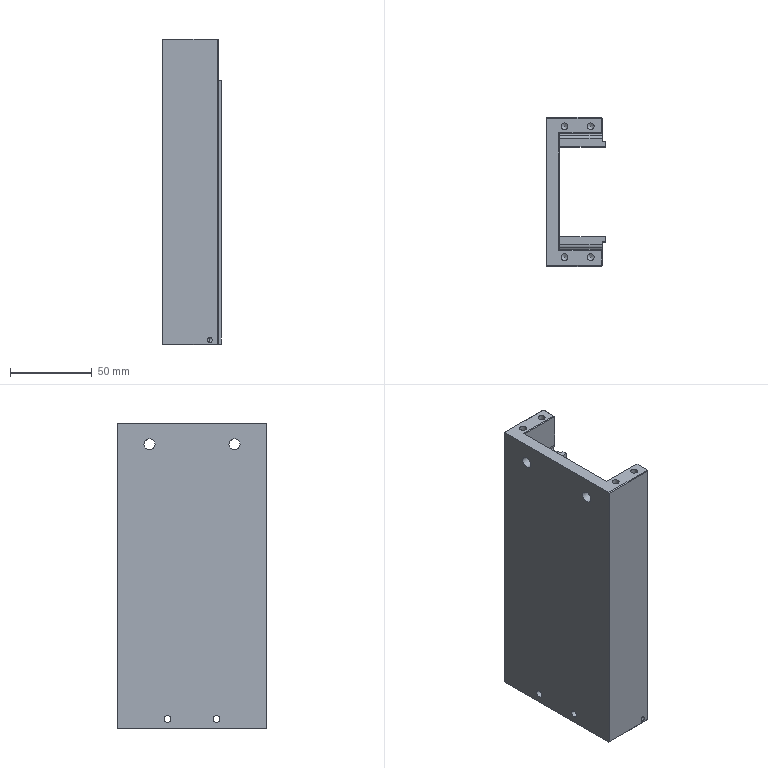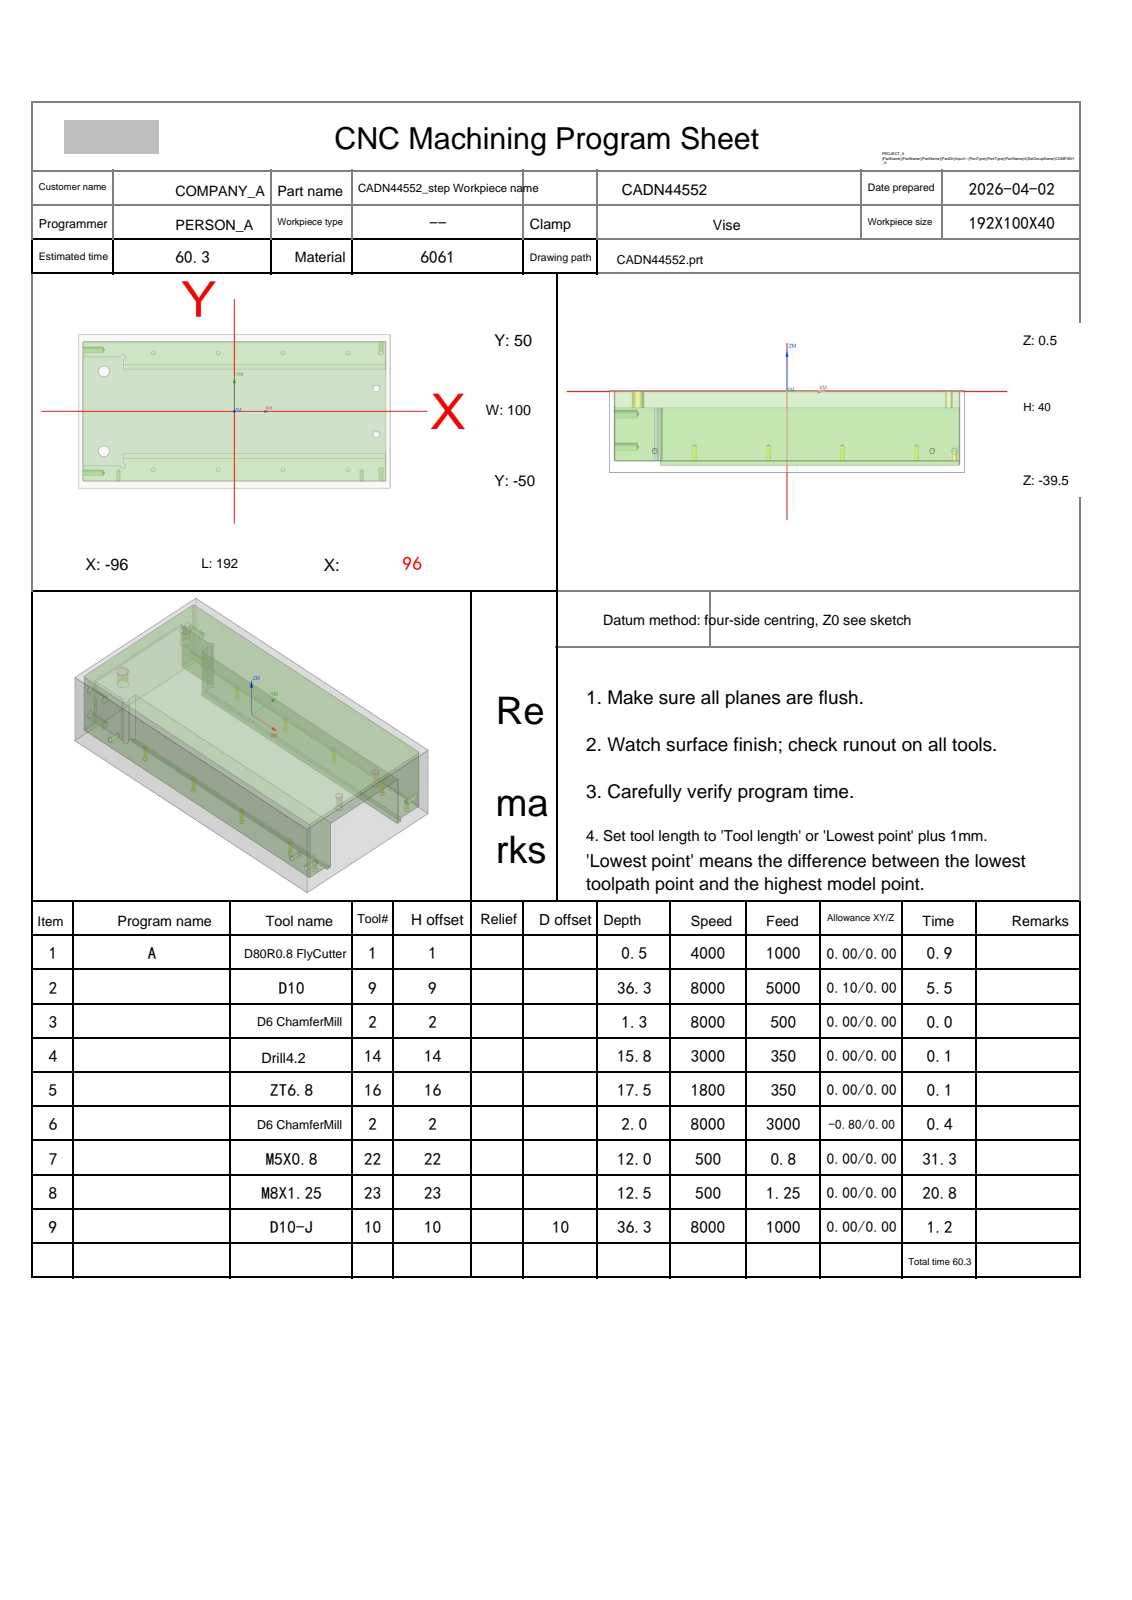NC program | NX | posted by the shop | part box 36 x 91 x 187 mm
Whole program:
%
O0001
(Machine time: 110.14 MIN)
(===Total Tool:8===)
(T1=D80R0.8 FlyCutter D=80.  R=0.8  D-  H01 Z=-0.   )
(T9=D10     D=10.  R=0.   D-  H09 Z=-35.8 )
(T2=D6 ChamferMill   D=6.   R=0.   D-  H02 Z=-1.5  )
(T14=Drill 4.2  D=4.2  DR_a=118 D-  H14 Z=-15.26)
(T16=ZT6.8  D=6.8  DR_a=118 D-  H16 Z=-17.04)
(T22=M5X0.8 D=4.2  DR_a=180 D-  H22 Z=-11.5 )
(T23=M8X1.25 D=6.8  DR_a=180 D-  H23 Z=-12.  )
(T10=D10-J  D=10.  R=0.   D10 H10 Z=-35.8 )
G80 G90 G17 G49 G40
G91 G28 Z0
M01
N1 T01 M06
(D80R0.8 FlyCutter  D=80. R=0.8 H=01 ce=0.00 di=0.00)
G00 G90 G54 X138.5 Y-42.75 M03 S4000
G43 H01 Z20.
M08
Z2.
G01 Z0.0 F1000.
X133.5
X-133.5
Y0.0
X133.5
Y42.75
X-133.5
X-138.5
Z2.
G00 Z20.
G91 G28 Z0.0
M05
M09
G91 G28 Z0.0
M01
N2 T09 M06
(D10  D=10. R=0. H=09 ce=0.10 di=0.00)
G00 G90 G54 X0.0 Y-50.6 M03 S8000
G43 H09 Z20.
M08
Z.5
G01 X-93. Z.375 F5000.
G02 X-96.606 Y-49.106 Z.37 I0.0 J5.1
G01 X-97.106 Y-48.606 Z.369
G02 X-98.6 Y-45. Z.363 I3.606 J3.606
G01 Y45. Z.242
G02 X-97.106 Y48.606 Z.237 I5.1 J0.0
G01 X-96.606 Y49.106 Z.236
G02 X-93. Y50.6 Z.23 I3.606 J-3.606
G01 X93. Z-.02
G02 X96.606 Y49.106 Z-.025 I0.0 J-5.1
G01 X97.106 Y48.606 Z-.026
G02 X98.6 Y45. Z-.031 I-3.606 J-3.606
G01 Y-45. Z-.152
G02 X97.106 Y-48.606 Z-.158 I-5.1 J0.0
G01 X96.606 Y-49.106 Z-.159
G02 X93. Y-50.6 Z-.164 I-3.606 J3.606
G01 X-93. Z-.414
G02 X-96.606 Y-49.106 Z-.42 I0.0 J5.1
G01 X-97.106 Y-48.606 Z-.421
G02 X-98.6 Y-45. Z-.426 I3.606 J3.606
G01 Y45. Z-.547
G02 X-97.106 Y48.606 Z-.552 I5.1 J0.0
G01 X-96.606 Y49.106 Z-.553
G02 X-93. Y50.6 Z-.559 I3.606 J-3.606
G01 X93. Z-.809
G02 X96.606 Y49.106 Z-.814 I0.0 J-5.1
G01 X97.106 Y48.606 Z-.815
G02 X98.6 Y45. Z-.82 I-3.606 J-3.606
G01 Y-45. Z-.941
G02 X97.106 Y-48.606 Z-.947 I-5.1 J0.0
G01 X96.606 Y-49.106 Z-.948
G02 X93. Y-50.6 Z-.953 I-3.606 J3.606
G01 X-93. Z-1.203
G02 X-96.606 Y-49.106 Z-1.209 I0.0 J5.1
G01 X-97.106 Y-48.606 Z-1.21
G02 X-98.6 Y-45. Z-1.215 I3.606 J3.606
G01 Y45. Z-1.336
G02 X-97.106 Y48.606 Z-1.341 I5.1 J0.0
G01 X-96.606 Y49.106 Z-1.342
G02 X-93. Y50.6 Z-1.348 I3.606 J-3.606
G01 X93. Z-1.598
G02 X96.606 Y49.106 Z-1.603 I0.0 J-5.1
G01 X97.106 Y48.606 Z-1.604
G02 X98.6 Y45. Z-1.61 I-3.606 J-3.606
G01 Y-45. Z-1.731
G02 X97.106 Y-48.606 Z-1.736 I-5.1 J0.0
G01 X96.606 Y-49.106 Z-1.737
G02 X93. Y-50.6 Z-1.742 I-3.606 J3.606
G01 X-93. Z-1.992
G02 X-96.606 Y-49.106 Z-1.998 I0.0 J5.1
G01 X-97.106 Y-48.606 Z-1.999
G02 X-98.6 Y-45. Z-2.004 I3.606 J3.606
G01 Y45. Z-2.125
G02 X-97.106 Y48.606 Z-2.131 I5.1 J0.0
G01 X-96.606 Y49.106 Z-2.132
G02 X-93. Y50.6 Z-2.137 I3.606 J-3.606
G01 X93. Z-2.387
G02 X96.606 Y49.106 Z-2.392 I0.0 J-5.1
G01 X97.106 Y48.606 Z-2.393
G02 X98.6 Y45. Z-2.399 I-3.606 J-3.606
G01 Y-45. Z-2.52
G02 X97.106 Y-48.606 Z-2.525 I-5.1 J0.0
G01 X96.606 Y-49.106 Z-2.526
G02 X93. Y-50.6 Z-2.531 I-3.606 J3.606
G01 X-93. Z-2.782
G02 X-96.606 Y-49.106 Z-2.787 I0.0 J5.1
G01 X-97.106 Y-48.606 Z-2.788
G02 X-98.6 Y-45. Z-2.793 I3.606 J3.606
G01 Y45. Z-2.914
G02 X-97.106 Y48.606 Z-2.92 I5.1 J0.0
G01 X-96.606 Y49.106 Z-2.921
G02 X-93. Y50.6 Z-2.926 I3.606 J-3.606
G01 X93. Z-3.176
G02 X96.606 Y49.106 Z-3.182 I0.0 J-5.1
G01 X97.106 Y48.606
G02 X98.6 Y45. Z-3.188 I-3.606 J-3.606
G01 Y-45. Z-3.309
G02 X97.106 Y-48.606 Z-3.314 I-5.1 J0.0
G01 X96.606 Y-49.106 Z-3.315
G02 X93. Y-50.6 Z-3.321 I-3.606 J3.606
G01 X-93. Z-3.571
G02 X-96.606 Y-49.106 Z-3.576 I0.0 J5.1
G01 X-97.106 Y-48.606 Z-3.577
G02 X-98.6 Y-45. Z-3.582 I3.606 J3.606
G01 Y45. Z-3.703
G02 X-97.106 Y48.606 Z-3.709 I5.1 J0.0
G01 X-96.606 Y49.106 Z-3.71
G02 X-93. Y50.6 Z-3.715 I3.606 J-3.606
G01 X93. Z-3.965
G02 X96.606 Y49.106 Z-3.971 I0.0 J-5.1
G01 X97.106 Y48.606 Z-3.972
G02 X98.6 Y45. Z-3.977 I-3.606 J-3.606
G01 Y-45. Z-4.098
G02 X97.106 Y-48.606 Z-4.103 I-5.1 J0.0
G01 X96.606 Y-49.106 Z-4.104
G02 X93. Y-50.6 Z-4.11 I-3.606 J3.606
G01 X-93. Z-4.36
G02 X-96.606 Y-49.106 Z-4.365 I0.0 J5.1
G01 X-97.106 Y-48.606 Z-4.366
G02 X-98.6 Y-45. Z-4.372 I3.606 J3.606
G01 Y45. Z-4.493
G02 X-97.106 Y48.606 Z-4.498 I5.1 J0.0
G01 X-96.606 Y49.106 Z-4.499
G02 X-93. Y50.6 Z-4.504 I3.606 J-3.606
G01 X93. Z-4.754
G02 X96.606 Y49.106 Z-4.76 I0.0 J-5.1
G01 X97.106 Y48.606 Z-4.761
G02 X98.6 Y45. Z-4.766 I-3.606 J-3.606
G01 Y-45. Z-4.887
G02 X97.106 Y-48.606 Z-4.893 I-5.1 J0.0
G01 X96.606 Y-49.106
G02 X93. Y-50.6 Z-4.899 I-3.606 J3.606
G01 X-93. Z-5.149
G02 X-96.606 Y-49.106 Z-5.154 I0.0 J5.1
G01 X-97.106 Y-48.606 Z-5.155
G02 X-98.6 Y-45. Z-5.161 I3.606 J3.606
G01 Y45. Z-5.282
G02 X-97.106 Y48.606 Z-5.287 I5.1 J0.0
G01 X-96.606 Y49.106 Z-5.288
G02 X-93. Y50.6 Z-5.293 I3.606 J-3.606
G01 X93. Z-5.544
G02 X96.606 Y49.106 Z-5.549 I0.0 J-5.1
G01 X97.106 Y48.606 Z-5.55
G02 X98.6 Y45. Z-5.555 I-3.606 J-3.606
G01 Y-45. Z-5.676
G02 X97.106 Y-48.606 Z-5.682 I-5.1 J0.0
G01 X96.606 Y-49.106 Z-5.683
G02 X93. Y-50.6 Z-5.688 I-3.606 J3.606
G01 X-93. Z-5.938
G02 X-96.606 Y-49.106 Z-5.943 I0.0 J5.1
G01 X-97.106 Y-48.606 Z-5.944
G02 X-98.6 Y-45. Z-5.95 I3.606 J3.606
G01 Y45. Z-6.071
G02 X-97.106 Y48.606 Z-6.076 I5.1 J0.0
G01 X-96.606 Y49.106 Z-6.077
G02 X-93. Y50.6 Z-6.083 I3.606 J-3.606
G01 X93. Z-6.333
G02 X96.606 Y49.106 Z-6.338 I0.0 J-5.1
G01 X97.106 Y48.606 Z-6.339
G02 X98.6 Y45. Z-6.344 I-3.606 J-3.606
G01 Y-45. Z-6.465
G02 X97.106 Y-48.606 Z-6.471 I-5.1 J0.0
G01 X96.606 Y-49.106 Z-6.472
G02 X93. Y-50.6 Z-6.477 I-3.606 J3.606
G01 X-93. Z-6.727
G02 X-96.606 Y-49.106 Z-6.733 I0.0 J5.1
G01 X-97.106 Y-48.606 Z-6.734
G02 X-98.6 Y-45. Z-6.739 I3.606 J3.606
G01 Y45. Z-6.86
G02 X-97.106 Y48.606 Z-6.865 I5.1 J0.0
G01 X-96.606 Y49.106 Z-6.866
G02 X-93. Y50.6 Z-6.872 I3.606 J-3.606
G01 X93. Z-7.122
G02 X96.606 Y49.106 Z-7.127 I0.0 J-5.1
G01 X97.106 Y48.606 Z-7.128
G02 X98.6 Y45. Z-7.134 I-3.606 J-3.606
G01 Y-45. Z-7.255
G02 X97.106 Y-48.606 Z-7.26 I-5.1 J0.0
G01 X96.606 Y-49.106 Z-7.261
G02 X93. Y-50.6 Z-7.266 I-3.606 J3.606
G01 X-93. Z-7.516
G02 X-96.606 Y-49.106 Z-7.522 I0.0 J5.1
G01 X-97.106 Y-48.606 Z-7.523
G02 X-98.6 Y-45. Z-7.528 I3.606 J3.606
G01 Y45. Z-7.649
G02 X-97.106 Y48.606 Z-7.654 I5.1 J0.0
G01 X-96.606 Y49.106 Z-7.655
G02 X-93. Y50.6 Z-7.661 I3.606 J-3.606
G01 X93. Z-7.911
G02 X96.606 Y49.106 Z-7.916 I0.0 J-5.1
G01 X97.106 Y48.606 Z-7.917
G02 X98.6 Y45. Z-7.923 I-3.606 J-3.606
G01 Y-45. Z-8.044
G02 X97.106 Y-48.606 Z-8.049 I-5.1 J0.0
G01 X96.606 Y-49.106 Z-8.05
G02 X93. Y-50.6 Z-8.055 I-3.606 J3.606
G01 X-93. Z-8.305
G02 X-96.606 Y-49.106 Z-8.311 I0.0 J5.1
G01 X-97.106 Y-48.606 Z-8.312
G02 X-98.6 Y-45. Z-8.317 I3.606 J3.606
G01 Y45. Z-8.438
G02 X-97.106 Y48.606 Z-8.444 I5.1 J0.0
G01 X-96.606 Y49.106 Z-8.445
G02 X-93. Y50.6 Z-8.45 I3.606 J-3.606
G01 X93. Z-8.7
G02 X96.606 Y49.106 Z-8.705 I0.0 J-5.1
G01 X97.106 Y48.606 Z-8.706
G02 X98.6 Y45. Z-8.712 I-3.606 J-3.606
G01 Y-45. Z-8.833
G02 X97.106 Y-48.606 Z-8.838 I-5.1 J0.0
G01 X96.606 Y-49.106 Z-8.839
G02 X93. Y-50.6 Z-8.845 I-3.606 J3.606
G01 X-93. Z-9.095
G02 X-96.606 Y-49.106 Z-9.1 I0.0 J5.1
G01 X-97.106 Y-48.606 Z-9.101
G02 X-98.6 Y-45. Z-9.106 I3.606 J3.606
G01 Y45. Z-9.227
G02 X-97.106 Y48.606 Z-9.233 I5.1 J0.0
G01 X-96.606 Y49.106 Z-9.234
G02 X-93. Y50.6 Z-9.239 I3.606 J-3.606
G01 X93. Z-9.489
G02 X96.606 Y49.106 Z-9.495 I0.0 J-5.1
G01 X97.106 Y48.606 Z-9.496
G02 X98.6 Y45. Z-9.501 I-3.606 J-3.606
G01 Y-45. Z-9.622
G02 X97.106 Y-48.606 Z-9.627 I-5.1 J0.0
G01 X96.606 Y-49.106 Z-9.628
G02 X93. Y-50.6 Z-9.634 I-3.606 J3.606
G01 X-93. Z-9.884
G02 X-96.606 Y-49.106 Z-9.889 I0.0 J5.1
G01 X-97.106 Y-48.606 Z-9.89
G02 X-98.6 Y-45. Z-9.895 I3.606 J3.606
G01 Y45. Z-10.016
G02 X-97.106 Y48.606 Z-10.022 I5.1 J0.0
G01 X-96.606 Y49.106 Z-10.023
G02 X-93. Y50.6 Z-10.028 I3.606 J-3.606
G01 X93. Z-10.278
G02 X96.606 Y49.106 Z-10.284 I0.0 J-5.1
G01 X97.106 Y48.606 Z-10.285
G02 X98.6 Y45. Z-10.29 I-3.606 J-3.606
G01 Y-45. Z-10.411
G02 X97.106 Y-48.606 Z-10.416 I-5.1 J0.0
G01 X96.606 Y-49.106 Z-10.417
G02 X93. Y-50.6 Z-10.423 I-3.606 J3.606
G01 X-93. Z-10.673
G02 X-96.606 Y-49.106 Z-10.678 I0.0 J5.1
G01 X-97.106 Y-48.606 Z-10.679
G02 X-98.6 Y-45. Z-10.685 I3.606 J3.606
G01 Y45. Z-10.806
G02 X-97.106 Y48.606 Z-10.811 I5.1 J0.0
G01 X-96.606 Y49.106 Z-10.812
G02 X-93. Y50.6 Z-10.817 I3.606 J-3.606
G01 X93. Z-11.067
G02 X96.606 Y49.106 Z-11.073 I0.0 J-5.1
G01 X97.106 Y48.606 Z-11.074
G02 X98.6 Y45. Z-11.079 I-3.606 J-3.606
G01 Y-45. Z-11.2
G02 X97.106 Y-48.606 Z-11.206 I-5.1 J0.0
G01 X96.606 Y-49.106 Z-11.207
G02 X93. Y-50.6 Z-11.212 I-3.606 J3.606
G01 X-93. Z-11.462
G02 X-96.606 Y-49.106 Z-11.467 I0.0 J5.1
G01 X-97.106 Y-48.606 Z-11.468
G02 X-98.6 Y-45. Z-11.474 I3.606 J3.606
G01 Y45. Z-11.595
G02 X-97.106 Y48.606 Z-11.6 I5.1 J0.0
G01 X-96.606 Y49.106 Z-11.601
G02 X-93. Y50.6 Z-11.606 I3.606 J-3.606
G01 X93. Z-11.857
G02 X96.606 Y49.106 Z-11.862 I0.0 J-5.1
G01 X97.106 Y48.606 Z-11.863
G02 X98.6 Y45. Z-11.868 I-3.606 J-3.606
G01 Y-45. Z-11.989
G02 X97.106 Y-48.606 Z-11.995 I-5.1 J0.0
G01 X96.606 Y-49.106 Z-11.996
G02 X93. Y-50.6 Z-12.001 I-3.606 J3.606
G01 X-93. Z-12.251
G02 X-96.606 Y-49.106 Z-12.257 I0.0 J5.1
G01 X-97.106 Y-48.606
G02 X-98.6 Y-45. Z-12.263 I3.606 J3.606
G01 Y45. Z-12.384
G02 X-97.106 Y48.606 Z-12.389 I5.1 J0.0
G01 X-96.606 Y49.106 Z-12.39
G02 X-93. Y50.6 Z-12.396 I3.606 J-3.606
G01 X93. Z-12.646
G02 X96.606 Y49.106 Z-12.651 I0.0 J-5.1
G01 X97.106 Y48.606 Z-12.652
G02 X98.6 Y45. Z-12.657 I-3.606 J-3.606
G01 Y-45. Z-12.778
G02 X97.106 Y-48.606 Z-12.784 I-5.1 J0.0
G01 X96.606 Y-49.106 Z-12.785
G02 X93. Y-50.6 Z-12.79 I-3.606 J3.606
G01 X-93. Z-13.04
G02 X-96.606 Y-49.106 Z-13.046 I0.0 J5.1
G01 X-97.106 Y-48.606 Z-13.047
G02 X-98.6 Y-45. Z-13.052 I3.606 J3.606
G01 Y45. Z-13.173
G02 X-97.106 Y48.606 Z-13.178 I5.1 J0.0
G01 X-96.606 Y49.106 Z-13.179
G02 X-93. Y50.6 Z-13.185 I3.606 J-3.606
G01 X93. Z-13.435
G02 X96.606 Y49.106 Z-13.44 I0.0 J-5.1
G01 X97.106 Y48.606 Z-13.441
G02 X98.6 Y45. Z-13.447 I-3.606 J-3.606
G01 Y-45. Z-13.568
G02 X97.106 Y-48.606 Z-13.573 I-5.1 J0.0
G01 X96.606 Y-49.106 Z-13.574
G02 X93. Y-50.6 Z-13.579 I-3.606 J3.606
G01 X-93. Z-13.829
G02 X-96.606 Y-49.106 Z-13.835 I0.0 J5.1
G01 X-97.106 Y-48.606 Z-13.836
G02 X-98.6 Y-45. Z-13.841 I3.606 J3.606
G01 Y45. Z-13.962
G02 X-97.106 Y48.606 Z-13.968 I5.1 J0.0
G01 X-96.606 Y49.106
G02 X-93. Y50.6 Z-13.974 I3.606 J-3.606
G01 X93. Z-14.224
G02 X96.606 Y49.106 Z-14.229 I0.0 J-5.1
G01 X97.106 Y48.606 Z-14.23
G02 X98.6 Y45. Z-14.236 I-3.606 J-3.606
G01 Y-45. Z-14.357
G02 X97.106 Y-48.606 Z-14.362 I-5.1 J0.0
G01 X96.606 Y-49.106 Z-14.363
G02 X93. Y-50.6 Z-14.368 I-3.606 J3.606
G01 X-93. Z-14.619
G02 X-96.606 Y-49.106 Z-14.624 I0.0 J5.1
G01 X-97.106 Y-48.606 Z-14.625
G02 X-98.6 Y-45. Z-14.63 I3.606 J3.606
G01 Y45. Z-14.751
G02 X-97.106 Y48.606 Z-14.757 I5.1 J0.0
G01 X-96.606 Y49.106 Z-14.758
G02 X-93. Y50.6 Z-14.763 I3.606 J-3.606
G01 X93. Z-15.013
G02 X96.606 Y49.106 Z-15.018 I0.0 J-5.1
G01 X97.106 Y48.606 Z-15.019
G02 X98.6 Y45. Z-15.025 I-3.606 J-3.606
G01 Y-45. Z-15.146
G02 X97.106 Y-48.606 Z-15.151 I-5.1 J0.0
G01 X96.606 Y-49.106 Z-15.152
G02 X93. Y-50.6 Z-15.158 I-3.606 J3.606
G01 X-93. Z-15.408
G02 X-96.606 Y-49.106 Z-15.413 I0.0 J5.1
G01 X-97.106 Y-48.606 Z-15.414
G02 X-98.6 Y-45. Z-15.419 I3.606 J3.606
G01 Y45. Z-15.54
G02 X-97.106 Y48.606 Z-15.546 I5.1 J0.0
G01 X-96.606 Y49.106 Z-15.547
G02 X-93. Y50.6 Z-15.552 I3.606 J-3.606
G01 X93. Z-15.802
G02 X96.606 Y49.106 Z-15.808 I0.0 J-5.1
G01 X97.106 Y48.606 Z-15.809
G02 X98.6 Y45. Z-15.814 I-3.606 J-3.606
G01 Y-45. Z-15.935
G02 X97.106 Y-48.606 Z-15.94 I-5.1 J0.0
G01 X96.606 Y-49.106 Z-15.941
G02 X93. Y-50.6 Z-15.947 I-3.606 J3.606
G01 X-93. Z-16.197
G02 X-96.606 Y-49.106 Z-16.202 I0.0 J5.1
G01 X-97.106 Y-48.606 Z-16.203
G02 X-98.6 Y-45. Z-16.209 I3.606 J3.606
G01 Y45. Z-16.33
G02 X-97.106 Y48.606 Z-16.335 I5.1 J0.0
G01 X-96.606 Y49.106 Z-16.336
G02 X-93. Y50.6 Z-16.341 I3.606 J-3.606
G01 X93. Z-16.591
G02 X96.606 Y49.106 Z-16.597 I0.0 J-5.1
G01 X97.106 Y48.606 Z-16.598
G02 X98.6 Y45. Z-16.603 I-3.606 J-3.606
G01 Y-45. Z-16.724
G02 X97.106 Y-48.606 Z-16.729 I-5.1 J0.0
G01 X96.606 Y-49.106 Z-16.73
G02 X93. Y-50.6 Z-16.736 I-3.606 J3.606
G01 X-93. Z-16.986
G02 X-96.606 Y-49.106 Z-16.991 I0.0 J5.1
G01 X-97.106 Y-48.606 Z-16.992
G02 X-98.6 Y-45. Z-16.998 I3.606 J3.606
G01 Y45. Z-17.119
G02 X-97.106 Y48.606 Z-17.124 I5.1 J0.0
G01 X-96.606 Y49.106 Z-17.125
G02 X-93. Y50.6 Z-17.13 I3.606 J-3.606
G01 X93. Z-17.38
G02 X96.606 Y49.106 Z-17.386 I0.0 J-5.1
G01 X97.106 Y48.606 Z-17.387
G02 X98.6 Y45. Z-17.392 I-3.606 J-3.606
G01 Y-45. Z-17.513
G02 X97.106 Y-48.606 Z-17.519 I-5.1 J0.0
G01 X96.606 Y-49.106 Z-17.52
G02 X93. Y-50.6 Z-17.525 I-3.606 J3.606
G01 X-93. Z-17.775
G02 X-96.606 Y-49.106 Z-17.78 I0.0 J5.1
G01 X-97.106 Y-48.606 Z-17.781
G02 X-98.6 Y-45. Z-17.787 I3.606 J3.606
G01 Y45. Z-17.908
G02 X-97.106 Y48.606 Z-17.913 I5.1 J0.0
G01 X-96.606 Y49.106 Z-17.914
G02 X-93. Y50.6 Z-17.92 I3.606 J-3.606
G01 X93. Z-18.17
G02 X96.606 Y49.106 Z-18.175 I0.0 J-5.1
G01 X97.106 Y48.606 Z-18.176
G02 X98.6 Y45. Z-18.181 I-3.606 J-3.606
G01 Y-45. Z-18.302
G02 X97.106 Y-48.606 Z-18.308 I-5.1 J0.0
G01 X96.606 Y-49.106 Z-18.309
G02 X93. Y-50.6 Z-18.314 I-3.606 J3.606
G01 X-93. Z-18.564
G02 X-96.606 Y-49.106 Z-18.57 I0.0 J5.1
G01 X-97.106 Y-48.606 Z-18.571
G02 X-98.6 Y-45. Z-18.576 I3.606 J3.606
G01 Y45. Z-18.697
G02 X-97.106 Y48.606 Z-18.702 I5.1 J0.0
G01 X-96.606 Y49.106 Z-18.703
G02 X-93. Y50.6 Z-18.709 I3.606 J-3.606
G01 X93. Z-18.959
G02 X96.606 Y49.106 Z-18.964 I0.0 J-5.1
G01 X97.106 Y48.606 Z-18.965
G02 X98.6 Y45. Z-18.97 I-3.606 J-3.606
G01 Y-45. Z-19.091
G02 X97.106 Y-48.606 Z-19.097 I-5.1 J0.0
G01 X96.606 Y-49.106 Z-19.098
G02 X93. Y-50.6 Z-19.103 I-3.606 J3.606
G01 X-93. Z-19.353
G02 X-96.606 Y-49.106 Z-19.359 I0.0 J5.1
G01 X-97.106 Y-48.606 Z-19.36
G02 X-98.6 Y-45. Z-19.365 I3.606 J3.606
G01 Y45. Z-19.486
G02 X-97.106 Y48.606 Z-19.491 I5.1 J0.0
G01 X-96.606 Y49.106 Z-19.492
G02 X-93. Y50.6 Z-19.498 I3.606 J-3.606
G01 X93. Z-19.748
G02 X96.606 Y49.106 Z-19.753 I0.0 J-5.1
G01 X97.106 Y48.606 Z-19.754
G02 X98.6 Y45. Z-19.76 I-3.606 J-3.606
G01 Y-45. Z-19.881
G02 X97.106 Y-48.606 Z-19.886 I-5.1 J0.0
G01 X96.606 Y-49.106 Z-19.887
G02 X93. Y-50.6 Z-19.892 I-3.606 J3.606
G01 X-93. Z-20.142
G02 X-96.606 Y-49.106 Z-20.148 I0.0 J5.1
G01 X-97.106 Y-48.606 Z-20.149
G02 X-98.6 Y-45. Z-20.154 I3.606 J3.606
G01 Y45. Z-20.275
G02 X-97.106 Y48.606 Z-20.281 I5.1 J0.0
G01 X-96.606 Y49.106 Z-20.282
G02 X-93. Y50.6 Z-20.287 I3.606 J-3.606
G01 X93. Z-20.537
G02 X96.606 Y49.106 Z-20.542 I0.0 J-5.1
G01 X97.106 Y48.606 Z-20.543
G02 X98.6 Y45. Z-20.549 I-3.606 J-3.606
G01 Y-45. Z-20.67
G02 X97.106 Y-48.606 Z-20.675 I-5.1 J0.0
G01 X96.606 Y-49.106 Z-20.676
G02 X93. Y-50.6 Z-20.681 I-3.606 J3.606
G01 X-93. Z-20.932
G02 X-96.606 Y-49.106 Z-20.937 I0.0 J5.1
G01 X-97.106 Y-48.606 Z-20.938
G02 X-98.6 Y-45. Z-20.943 I3.606 J3.606
G01 Y45. Z-21.064
G02 X-97.106 Y48.606 Z-21.07 I5.1 J0.0
G01 X-96.606 Y49.106 Z-21.071
G02 X-93. Y50.6 Z-21.076 I3.606 J-3.606
G01 X93. Z-21.326
G02 X96.606 Y49.106 Z-21.332 I0.0 J-5.1
G01 X97.106 Y48.606
G02 X98.6 Y45. Z-21.338 I-3.606 J-3.606
G01 Y-45. Z-21.459
G02 X97.106 Y-48.606 Z-21.464 I-5.1 J0.0
G01 X96.606 Y-49.106 Z-21.465
G02 X93. Y-50.6 Z-21.471 I-3.606 J3.606
G01 X-93. Z-21.721
G02 X-96.606 Y-49.106 Z-21.726 I0.0 J5.1
G01 X-97.106 Y-48.606 Z-21.727
G02 X-98.6 Y-45. Z-21.732 I3.606 J3.606
G01 Y45. Z-21.853
G02 X-97.106 Y48.606 Z-21.859 I5.1 J0.0
G01 X-96.606 Y49.106 Z-21.86
G02 X-93. Y50.6 Z-21.865 I3.606 J-3.606
G01 X93. Z-22.115
G02 X96.606 Y49.106 Z-22.121 I0.0 J-5.1
G01 X97.106 Y48.606 Z-22.122
G02 X98.6 Y45. Z-22.127 I-3.606 J-3.606
G01 Y-45. Z-22.248
G02 X97.106 Y-48.606 Z-22.253 I-5.1 J0.0
G01 X96.606 Y-49.106 Z-22.254
G02 X93. Y-50.6 Z-22.26 I-3.606 J3.606
G01 X-93. Z-22.51
G02 X-96.606 Y-49.106 Z-22.515 I0.0 J5.1
G01 X-97.106 Y-48.606 Z-22.516
G02 X-98.6 Y-45. Z-22.522 I3.606 J3.606
G01 Y45. Z-22.643
G02 X-97.106 Y48.606 Z-22.648 I5.1 J0.0
G01 X-96.606 Y49.106 Z-22.649
G02 X-93. Y50.6 Z-22.654 I3.606 J-3.606
G01 X93. Z-22.904
G02 X96.606 Y49.106 Z-22.91 I0.0 J-5.1
G01 X97.106 Y48.606 Z-22.911
G02 X98.6 Y45. Z-22.916 I-3.606 J-3.606
G01 Y-45. Z-23.037
G02 X97.106 Y-48.606 Z-23.043 I-5.1 J0.0
G01 X96.606 Y-49.106
G02 X93. Y-50.6 Z-23.049 I-3.606 J3.606
G01 X-93. Z-23.299
G02 X-96.606 Y-49.106 Z-23.304 I0.0 J5.1
G01 X-97.106 Y-48.606 Z-23.305
G02 X-98.6 Y-45. Z-23.311 I3.606 J3.606
G01 Y45. Z-23.432
G02 X-97.106 Y48.606 Z-23.437 I5.1 J0.0
G01 X-96.606 Y49.106 Z-23.438
G02 X-93. Y50.6 Z-23.443 I3.606 J-3.606
G01 X93. Z-23.694
G02 X96.606 Y49.106 Z-23.699 I0.0 J-5.1
G01 X97.106 Y48.606 Z-23.7
G02 X98.6 Y45. Z-23.705 I-3.606 J-3.606
G01 Y-45. Z-23.826
G02 X97.106 Y-48.606 Z-23.832 I-5.1 J0.0
G01 X96.606 Y-49.106 Z-23.833
G02 X93. Y-50.6 Z-23.838 I-3.606 J3.606
G01 X-93. Z-24.088
G02 X-96.606 Y-49.106 Z-24.093 I0.0 J5.1
G01 X-97.106 Y-48.606 Z-24.094
G02 X-98.6 Y-45. Z-24.1 I3.606 J3.606
G01 Y45. Z-24.221
G02 X-97.106 Y48.606 Z-24.226 I5.1 J0.0
G01 X-96.606 Y49.106 Z-24.227
G02 X-93. Y50.6 Z-24.233 I3.606 J-3.606
G01 X93. Z-24.483
G02 X96.606 Y49.106 Z-24.488 I0.0 J-5.1
G01 X97.106 Y48.606 Z-24.489
G02 X98.6 Y45. Z-24.494 I-3.606 J-3.606
G01 Y-45. Z-24.615
G02 X97.106 Y-48.606 Z-24.621 I-5.1 J0.0
G01 X96.606 Y-49.106 Z-24.622
G02 X93. Y-50.6 Z-24.627 I-3.606 J3.606
G01 X-93. Z-24.877
G02 X-96.606 Y-49.106 Z-24.883 I0.0 J5.1
G01 X-97.106 Y-48.606 Z-24.884
G02 X-98.6 Y-45. Z-24.889 I3.606 J3.606
G01 Y45. Z-25.01
G02 X-97.106 Y48.606 Z-25.015 I5.1 J0.0
G01 X-96.606 Y49.106 Z-25.016
G02 X-93. Y50.6 Z-25.022 I3.606 J-3.606
G01 X93. Z-25.272
G02 X96.606 Y49.106 Z-25.277 I0.0 J-5.1
G01 X97.106 Y48.606 Z-25.278
G02 X98.6 Y45. Z-25.284 I-3.606 J-3.606
G01 Y-45. Z-25.405
G02 X97.106 Y-48.606 Z-25.41 I-5.1 J0.0
G01 X96.606 Y-49.106 Z-25.411
G02 X93. Y-50.6 Z-25.416 I-3.606 J3.606
G01 X-93. Z-25.666
G02 X-96.606 Y-49.106 Z-25.672 I0.0 J5.1
G01 X-97.106 Y-48.606 Z-25.673
G02 X-98.6 Y-45. Z-25.678 I3.606 J3.606
G01 Y45. Z-25.799
G02 X-97.106 Y48.606 Z-25.804 I5.1 J0.0
G01 X-96.606 Y49.106 Z-25.805
G02 X-93. Y50.6 Z-25.811 I3.606 J-3.606
G01 X93. Z-26.061
G02 X96.606 Y49.106 Z-26.066 I0.0 J-5.1
G01 X97.106 Y48.606 Z-26.067
G02 X98.6 Y45. Z-26.073 I-3.606 J-3.606
G01 Y-45. Z-26.194
G02 X97.106 Y-48.606 Z-26.199 I-5.1 J0.0
G01 X96.606 Y-49.106 Z-26.2
G02 X93. Y-50.6 Z-26.205 I-3.606 J3.606
G01 X-93. Z-26.455
G02 X-96.606 Y-49.106 Z-26.461 I0.0 J5.1
G01 X-97.106 Y-48.606 Z-26.462
G02 X-98.6 Y-45. Z-26.467 I3.606 J3.606
G01 Y45. Z-26.588
G02 X-97.106 Y48.606 Z-26.594 I5.1 J0.0
G01 X-96.606 Y49.106 Z-26.595
G02 X-93. Y50.6 Z-26.6 I3.606 J-3.606
G01 X93. Z-26.85
G02 X96.606 Y49.106 Z-26.855 I0.0 J-5.1
G01 X97.106 Y48.606 Z-26.856
G02 X98.6 Y45. Z-26.862 I-3.606 J-3.606
G01 Y-45. Z-26.983
G02 X97.106 Y-48.606 Z-26.988 I-5.1 J0.0
G01 X96.606 Y-49.106 Z-26.989
G02 X93. Y-50.6 Z-26.995 I-3.606 J3.606
G01 X-93. Z-27.245
G02 X-96.606 Y-49.106 Z-27.25 I0.0 J5.1
G01 X-97.106 Y-48.606 Z-27.251
G02 X-98.6 Y-45. Z-27.256 I3.606 J3.606
G01 Y45. Z-27.377
G02 X-97.106 Y48.606 Z-27.383 I5.1 J0.0
G01 X-96.606 Y49.106 Z-27.384
G02 X-93. Y50.6 Z-27.389 I3.606 J-3.606
G01 X93. Z-27.639
G02 X96.606 Y49.106 Z-27.645 I0.0 J-5.1
G01 X97.106 Y48.606 Z-27.646
G02 X98.6 Y45. Z-27.651 I-3.606 J-3.606
G01 Y-45. Z-27.772
G02 X97.106 Y-48.606 Z-27.777 I-5.1 J0.0
G01 X96.606 Y-49.106 Z-27.778
G02 X93. Y-50.6 Z-27.784 I-3.606 J3.606
G01 X-93. Z-28.034
G02 X-96.606 Y-49.106 Z-28.039 I0.0 J5.1
G01 X-97.106 Y-48.606 Z-28.04
G02 X-98.6 Y-45. Z-28.045 I3.606 J3.606
G01 Y45. Z-28.166
G02 X-97.106 Y48.606 Z-28.172 I5.1 J0.0
G01 X-96.606 Y49.106 Z-28.173
G02 X-93. Y50.6 Z-28.178 I3.606 J-3.606
G01 X93. Z-28.428
G02 X96.606 Y49.106 Z-28.434 I0.0 J-5.1
G01 X97.106 Y48.606 Z-28.435
G02 X98.6 Y45. Z-28.44 I-3.606 J-3.606
G01 Y-45. Z-28.561
G02 X97.106 Y-48.606 Z-28.566 I-5.1 J0.0
G01 X96.606 Y-49.106 Z-28.567
G02 X93. Y-50.6 Z-28.573 I-3.606 J3.606
G01 X-93. Z-28.823
G02 X-96.606 Y-49.106 Z-28.828 I0.0 J5.1
G01 X-97.106 Y-48.606 Z-28.829
G02 X-98.6 Y-45. Z-28.835 I3.606 J3.606
G01 Y45. Z-28.956
G02 X-97.106 Y48.606 Z-28.961 I5.1 J0.0
G01 X-96.606 Y49.106 Z-28.962
G02 X-93. Y50.6 Z-28.967 I3.606 J-3.606
G01 X93. Z-29.217
G02 X96.606 Y49.106 Z-29.223 I0.0 J-5.1
G01 X97.106 Y48.606 Z-29.224
G02 X98.6 Y45. Z-29.229 I-3.606 J-3.606
G01 Y-45. Z-29.35
G02 X97.106 Y-48.606 Z-29.356 I-5.1 J0.0
G01 X96.606 Y-49.106 Z-29.357
G02 X93. Y-50.6 Z-29.362 I-3.606 J3.606
G01 X-93. Z-29.612
G02 X-96.606 Y-49.106 Z-29.617 I0.0 J5.1
G01 X-97.106 Y-48.606 Z-29.618
G02 X-98.6 Y-45. Z-29.624 I3.606 J3.606
G01 Y45. Z-29.745
G02 X-97.106 Y48.606 Z-29.75 I5.1 J0.0
G01 X-96.606 Y49.106 Z-29.751
G02 X-93. Y50.6 Z-29.756 I3.606 J-3.606
G01 X93. Z-30.007
G02 X96.606 Y49.106 Z-30.012 I0.0 J-5.1
G01 X97.106 Y48.606 Z-30.013
G02 X98.6 Y45. Z-30.018 I-3.606 J-3.606
G01 Y-45. Z-30.139
G02 X97.106 Y-48.606 Z-30.145 I-5.1 J0.0
G01 X96.606 Y-49.106 Z-30.146
G02 X93. Y-50.6 Z-30.151 I-3.606 J3.606
G01 X-93. Z-30.401
G02 X-96.606 Y-49.106 Z-30.407 I0.0 J5.1
G01 X-97.106 Y-48.606
G02 X-98.6 Y-45. Z-30.413 I3.606 J3.606
G01 Y45. Z-30.534
G02 X-97.106 Y48.606 Z-30.539 I5.1 J0.0
G01 X-96.606 Y49.106 Z-30.54
G02 X-93. Y50.6 Z-30.546 I3.606 J-3.606
G01 X93. Z-30.796
G02 X96.606 Y49.106 Z-30.801 I0.0 J-5.1
G01 X97.106 Y48.606 Z-30.802
G02 X98.6 Y45. Z-30.807 I-3.606 J-3.606
G01 Y-45. Z-30.928
G02 X97.106 Y-48.606 Z-30.934 I-5.1 J0.0
G01 X96.606 Y-49.106 Z-30.935
G02 X93. Y-50.6 Z-30.94 I-3.606 J3.606
G01 X-93. Z-31.19
G02 X-96.606 Y-49.106 Z-31.196 I0.0 J5.1
G01 X-97.106 Y-48.606 Z-31.197
G02 X-98.6 Y-45. Z-31.202 I3.606 J3.606
G01 Y45. Z-31.323
G02 X-97.106 Y48.606 Z-31.328 I5.1 J0.0
G01 X-96.606 Y49.106 Z-31.329
G02 X-93. Y50.6 Z-31.335 I3.606 J-3.606
G01 X93. Z-31.585
G02 X96.606 Y49.106 Z-31.59 I0.0 J-5.1
G01 X97.106 Y48.606 Z-31.591
G02 X98.6 Y45. Z-31.597 I-3.606 J-3.606
G01 Y-45. Z-31.718
G02 X97.106 Y-48.606 Z-31.723 I-5.1 J0.0
G01 X96.606 Y-49.106 Z-31.724
G02 X93. Y-50.6 Z-31.729 I-3.606 J3.606
G01 X-93. Z-31.979
G02 X-96.606 Y-49.106 Z-31.985 I0.0 J5.1
G01 X-97.106 Y-48.606 Z-31.986
G02 X-98.6 Y-45. Z-31.991 I3.606 J3.606
G01 Y45. Z-32.112
G02 X-97.106 Y48.606 Z-32.118 I5.1 J0.0
G01 X-96.606 Y49.106
G02 X-93. Y50.6 Z-32.124 I3.606 J-3.606
G01 X93. Z-32.374
G02 X96.606 Y49.106 Z-32.379 I0.0 J-5.1
G01 X97.106 Y48.606 Z-32.38
G02 X98.6 Y45. Z-32.386 I-3.606 J-3.606
G01 Y-45. Z-32.507
G02 X97.106 Y-48.606 Z-32.512 I-5.1 J0.0
G01 X96.606 Y-49.106 Z-32.513
G02 X93. Y-50.6 Z-32.518 I-3.606 J3.606
G01 X-93. Z-32.769
G02 X-96.606 Y-49.106 Z-32.774 I0.0 J5.1
G01 X-97.106 Y-48.606 Z-32.775
G02 X-98.6 Y-45. Z-32.78 I3.606 J3.606
G01 Y45. Z-32.901
G02 X-97.106 Y48.606 Z-32.907 I5.1 J0.0
G01 X-96.606 Y49.106 Z-32.908
G02 X-93. Y50.6 Z-32.913 I3.606 J-3.606
G01 X93. Z-33.163
G02 X96.606 Y49.106 Z-33.168 I0.0 J-5.1
G01 X97.106 Y48.606 Z-33.169
G02 X98.6 Y45. Z-33.175 I-3.606 J-3.606
G01 Y-45. Z-33.296
G02 X97.106 Y-48.606 Z-33.301 I-5.1 J0.0
G01 X96.606 Y-49.106 Z-33.302
G02 X93. Y-50.6 Z-33.308 I-3.606 J3.606
G01 X-93. Z-33.558
G02 X-96.606 Y-49.106 Z-33.563 I0.0 J5.1
G01 X-97.106 Y-48.606 Z-33.564
G02 X-98.6 Y-45. Z-33.569 I3.606 J3.606
G01 Y45. Z-33.69
G02 X-97.106 Y48.606 Z-33.696 I5.1 J0.0
G01 X-96.606 Y49.106 Z-33.697
G02 X-93. Y50.6 Z-33.702 I3.606 J-3.606
G01 X93. Z-33.952
G02 X96.606 Y49.106 Z-33.958 I0.0 J-5.1
G01 X97.106 Y48.606 Z-33.959
G02 X98.6 Y45. Z-33.964 I-3.606 J-3.606
G01 Y-45. Z-34.085
G02 X97.106 Y-48.606 Z-34.09 I-5.1 J0.0
G01 X96.606 Y-49.106 Z-34.091
G02 X93. Y-50.6 Z-34.097 I-3.606 J3.606
G01 X-93. Z-34.347
G02 X-96.606 Y-49.106 Z-34.352 I0.0 J5.1
G01 X-97.106 Y-48.606 Z-34.353
G02 X-98.6 Y-45. Z-34.359 I3.606 J3.606
G01 Y45. Z-34.48
G02 X-97.106 Y48.606 Z-34.485 I5.1 J0.0
G01 X-96.606 Y49.106 Z-34.486
G02 X-93. Y50.6 Z-34.491 I3.606 J-3.606
G01 X93. Z-34.741
G02 X96.606 Y49.106 Z-34.747 I0.0 J-5.1
G01 X97.106 Y48.606 Z-34.748
G02 X98.6 Y45. Z-34.753 I-3.606 J-3.606
G01 Y-45. Z-34.874
G02 X97.106 Y-48.606 Z-34.879 I-5.1 J0.0
G01 X96.606 Y-49.106 Z-34.88
G02 X93. Y-50.6 Z-34.886 I-3.606 J3.606
G01 X-93. Z-35.136
G02 X-96.606 Y-49.106 Z-35.141 I0.0 J5.1
G01 X-97.106 Y-48.606 Z-35.142
G02 X-98.6 Y-45. Z-35.148 I3.606 J3.606
G01 Y45. Z-35.269
G02 X-97.106 Y48.606 Z-35.274 I5.1 J0.0
G01 X-96.606 Y49.106 Z-35.275
G02 X-93. Y50.6 Z-35.28 I3.606 J-3.606
G01 X93. Z-35.53
G02 X96.606 Y49.106 Z-35.536 I0.0 J-5.1
G01 X97.106 Y48.606 Z-35.537
G02 X98.6 Y45. Z-35.542 I-3.606 J-3.606
G01 Y-45. Z-35.663
G02 X97.106 Y-48.606 Z-35.669 I-5.1 J0.0
G01 X96.606 Y-49.106 Z-35.67
G02 X93. Y-50.6 Z-35.675 I-3.606 J3.606
G01 X0.0 Z-35.8
X-93.
G02 X-96.606 Y-49.106 I0.0 J5.1
G01 X-97.106 Y-48.606
G02 X-98.6 Y-45. I3.606 J3.606
G01 Y45.
G02 X-97.106 Y48.606 I5.1 J0.0
G01 X-96.606 Y49.106
G02 X-93. Y50.6 I3.606 J-3.606
G01 X93.
G02 X96.606 Y49.106 I0.0 J-5.1
G01 X97.106 Y48.606
G02 X98.6 Y45. I-3.606 J-3.606
G01 Y-45.
G02 X97.106 Y-48.606 I-5.1 J0.0
G01 X96.606 Y-49.106
G02 X93. Y-50.6 I-3.606 J3.606
G01 X0.0
X-.5
Z-34.8
G00 Z20.
G91 G28 Z0.0
M05
M09
G91 G28 Z0.0
M01
N3 T02 M06
(D6 ChamferMill  D=6. R=0. H=02 ce=0.00 di=0.00)
G00 G90 G54 X87.5 Y-15. M03 S8000
G43 H02 Z20.
M08
G98 G81 X87.5 Y-15. Z-.8 R1. F500.
Y15.
X-80.5 Y26.
Y-26.
G80
G00 Z20.
G91 G28 Z0.0
M05
M09
G91 G28 Z0.0
M01
N4 T14 M06
(Drill 4.2 D=4.2 DR_a=118 H=14)
G00 G90 G54 X87.5 Y-15. M03 S3000
G43 H14 Z20.
M08
G98 G83 X87.5 Y-15. Z-15.262 R1. F350. Q3.
Y15.
G80
G00 Z20.
G91 G28 Z0.0
M05
M09
G91 G28 Z0.0
M01
N5 T16 M06
(ZT6.8 D=6.8 DR_a=118 H=16)
G00 G90 G54 X-80.5 Y26. M03 S1800
G43 H16 Z20.
M08
G98 G83 X-80.5 Y26. Z-17.043 R1. F350. Q3.
Y-26.
G80
G00 Z20.
G91 G28 Z0.0
M05
M09
G91 G28 Z0.0
M01
N6 T02 M06
(D6 ChamferMill  D=6. R=0. H=02 ce=0.00 di=0.00)
G00 G90 G54 X.25 Y-47.628 M03 S8000
G43 H02 Z20.
M08
Z2.099
G01 Z-1.5 F3000.
G03 X.33 Y-47.328 I-.52 J.3
X.03 Y-46.808 I-.6 J0.0
G01 X0.0 Y-46.8
X-93.
X-93.254 Y-46.775
X-93.497 Y-46.701
X-93.722 Y-46.581
X-93.919 Y-46.419
X-94.419 Y-45.919
X-94.581 Y-45.722
X-94.701 Y-45.497
X-94.775 Y-45.254
X-94.8 Y-45.
Y45.
X-94.775 Y45.254
X-94.701 Y45.497
X-94.581 Y45.722
X-94.419 Y45.919
X-93.919 Y46.419
X-93.722 Y46.581
X-93.497 Y46.701
X-93.254 Y46.775
X-93. Y46.8
X93.
X93.254 Y46.775
X93.497 Y46.701
X93.722 Y46.581
X93.919 Y46.419
X94.419 Y45.919
X94.581 Y45.722
X94.701 Y45.497
X94.775 Y45.254
X94.8 Y45.
Y-45.
X94.775 Y-45.254
X94.701 Y-45.497
X94.581 Y-45.722
X94.419 Y-45.919
X93.919 Y-46.419
X93.722 Y-46.581
X93.497 Y-46.701
X93.254 Y-46.775
X93. Y-46.8
X0.0
X-.03 Y-46.808
G03 X-.33 Y-47.328 I.3 J-.52
X-.25 Y-47.628 I.6 J0.0
G01 Z2.099
G00 Z20.
G00 G90 X87.593 Y-15.694 M03 S8000
Z20.
Z-.5
G01 Z-1. F500.
X87.7 Y-16.5
G03 X89.2 Y-15. I0.0 J1.5
X87.5 Y-13.3 I-1.7 J0.0
X85.8 Y-15. I0.0 J-1.7
X87.5 Y-16.7 I1.7 J0.0
X89.2 Y-15. I0.0 J1.7
X87.7 Y-13.5 I-1.5 J0.0
G01 X87.593 Y-14.306
Z-.5
G00 Z20.
Y14.306
Z-.5
G01 Z-1.
X87.7 Y13.5
G03 X89.2 Y15. I0.0 J1.5
X87.5 Y16.7 I-1.7 J0.0
X85.8 Y15. I0.0 J-1.7
X87.5 Y13.3 I1.7 J0.0
X89.2 Y15. I0.0 J1.7
X87.7 Y16.5 I-1.5 J0.0
G01 X87.593 Y15.694
Z-.5
G00 Z20.
G00 G90 X-81.666 Y27.5 M03 S8000
Z20.
Z-.8
G01 Z-1.3 F600.
X-81.9
G03 X-83.4 Y26. I0.0 J-1.5
X-80.5 Y23.1 I2.9 J0.0
X-77.6 Y26. I0.0 J2.9
X-80.5 Y28.9 I-2.9 J0.0
X-83.4 Y26. I0.0 J-2.9
X-81.9 Y24.5 I1.5 J0.0
G01 X-81.666
Z-.8
G00 Z20.
Y-24.5
Z-.8
G01 Z-1.3
X-81.9
G03 X-83.4 Y-26. I0.0 J-1.5
X-80.5 Y-28.9 I2.9 J0.0
X-77.6 Y-26. I0.0 J2.9
X-80.5 Y-23.1 I-2.9 J0.0
X-83.4 Y-26. I0.0 J-2.9
X-81.9 Y-27.5 I1.5 J0.0
G01 X-81.666
Z-.8
G00 Z20.
G91 G28 Z0.0
M05
M09
G91 G28 Z0.0
M01
N7 T22 M06
(M5X0.8 D=4.2 DR_a=180 H=22)
G00 G90 G54 X87.5 Y-15. M03 S500
G43 H22 Z20.
M08
G95
G98 G84 X87.5 Y-15. Z-11.5 R1. F.8 Q3.
Y15.
G80
G94
G00 Z20.
G91 G28 Z0.0
M05
M09
G91 G28 Z0.0
M01
N8 T23 M06
(M8X1.25 D=6.8 DR_a=180 H=23)
G00 G90 G54 X-80.5 Y26. M03 S500
G43 H23 Z20.
M08
G95
G98 G84 X-80.5 Y26. Z-12. R1. F1.25 Q4.
Y-26.
G80
G94
G00 Z20.
G91 G28 Z0.0
M05
M09
G91 G28 Z0.0
M01
N9 T10 M06
(D10-J  D=10. R=0. H=10 ce=0.00 di=0.00)
G00 G90 G54 X-94.013 Y51.616 M03 S8000
G43 H10 Z20.
M08
Z-17.4
G01 Z-17.9 F1000.
G41 D10
X-93.997 Y51.417
G03 X-93. Y50.5 I.997 J.083
G01 X93.
G02 X96.536 Y49.036 I0.0 J-5.
G01 X97.036 Y48.536
G02 X98.5 Y45. I-3.536 J-3.536
G01 Y-45.
G02 X97.036 Y-48.536 I-5. J0.0
G01 X96.536 Y-49.036
G02 X93. Y-50.5 I-3.536 J3.536
G01 X-93.
G02 X-96.536 Y-49.036 I0.0 J5.
G01 X-97.036 Y-48.536
G02 X-98.5 Y-45. I3.536 J3.536
G01 Y45.
G02 X-97.036 Y48.536 I5. J0.0
G01 X-96.536 Y49.036
G02 X-93. Y50.5 I3.536 J-3.536
G01 X-92.5
G03 X-91.5 Y51.5 I0.0 J1.
G01 G40 Y51.7
Z-17.4
G00 Z20.
X-94.013 Y51.616
Z-35.3
G01 Z-35.8
G41 D10
X-93.997 Y51.417
G03 X-93. Y50.5 I.997 J.083
G01 X93.
G02 X96.536 Y49.036 I0.0 J-5.
G01 X97.036 Y48.536
G02 X98.5 Y45. I-3.536 J-3.536
G01 Y-45.
G02 X97.036 Y-48.536 I-5. J0.0
G01 X96.536 Y-49.036
G02 X93. Y-50.5 I-3.536 J3.536
G01 X-93.
G02 X-96.536 Y-49.036 I0.0 J5.
G01 X-97.036 Y-48.536
G02 X-98.5 Y-45. I3.536 J3.536
G01 Y45.
G02 X-97.036 Y48.536 I5. J0.0
G01 X-96.536 Y49.036
G02 X-93. Y50.5 I3.536 J-3.536
G01 X-92.5
G03 X-91.5 Y51.5 I0.0 J1.
G01 G40 Y51.7
Z-35.3
G00 Z20.
M05
M09
G91 G28 Z0.0
G91 G28 Y0.0
M30
%